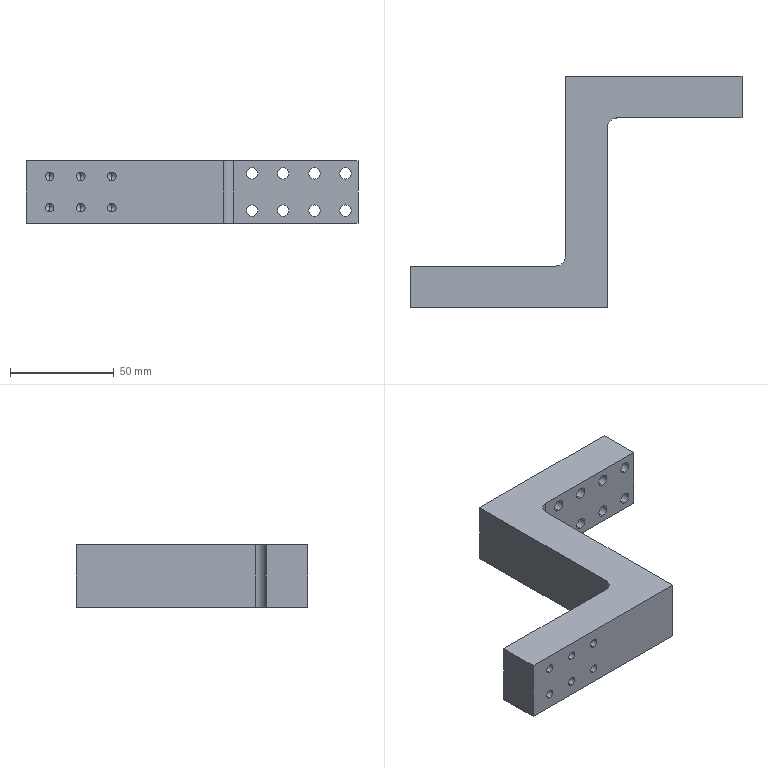Part | STEP file | ASND-0110-TPIM-065 | 1 solid | 52 faces | box 160 x 111.5 x 30 mm | volume 146139 mm3 | cylinder 30 | cone 12 | plane 10 | commonest cylinder face diameters 5.5 x16 4.2 x12 10 x2